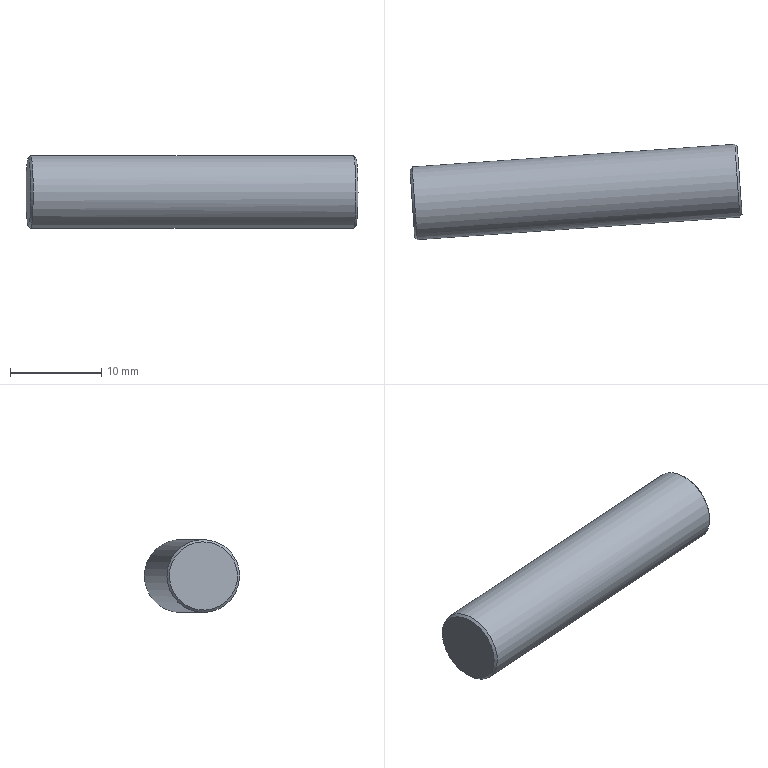Part | STEP file | 车灯-后视镜_id270_x_t | 1 solid | 5 faces | box 36.435 x 10.457 x 8 mm | volume 1807 mm3 | plane 2 | spline 2 | cylinder 1 | commonest cylinder face diameters 8 x1